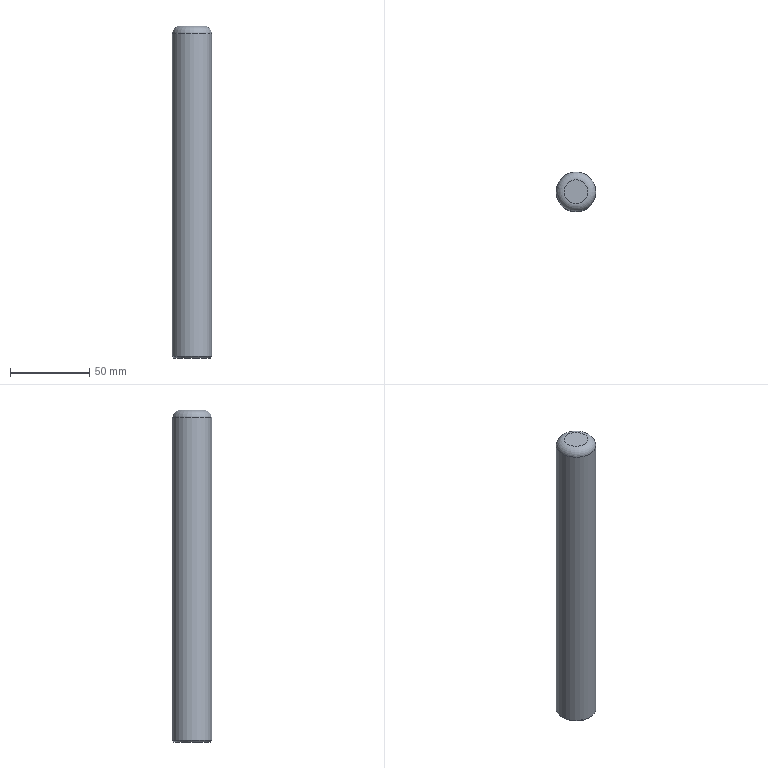Part | STEP file | 200 mesh_id66_xmt | 1 solid | 5 faces | box 25 x 25 x 210 mm | volume 102662 mm3 | plane 2 | cylinder 1 | cone 1 | torus 1 | commonest cylinder face diameters 25 x1
STEP:
#1=CARTESIAN_POINT('',(-17045.384,-4158.269,160.));
#2=VERTEX_POINT('',#1);
#3=CARTESIAN_POINT('',(-17052.884,-4158.269,160.));
#4=DIRECTION('',(0.,0.,1.));
#5=DIRECTION('',(1.,0.,0.));
#6=AXIS2_PLACEMENT_3D('',#3,#4,#5);
#7=CIRCLE('',#6,7.5);
#8=EDGE_CURVE('',#2,#2,#7,.T.);
#9=ORIENTED_EDGE('',*,*,#8,.T.);
#10=EDGE_LOOP('',(#9));
#11=FACE_OUTER_BOUND('',#10,.T.);
#12=CARTESIAN_POINT('',(-17052.884,-4158.269,160.));
#13=DIRECTION('',(0.,0.,1.));
#14=DIRECTION('',(1.,0.,0.));
#15=AXIS2_PLACEMENT_3D('',#12,#13,#14);
#16=PLANE('',#15);
#17=ADVANCED_FACE('',(#11),#16,.T.);
#18=CARTESIAN_POINT('',(-17064.384,-4158.269,-50.));
#19=VERTEX_POINT('',#18);
#20=CARTESIAN_POINT('',(-17052.884,-4158.269,-50.));
#21=DIRECTION('',(0.,0.,-1.));
#22=DIRECTION('',(-1.,0.,0.));
#23=AXIS2_PLACEMENT_3D('',#20,#21,#22);
#24=CIRCLE('',#23,11.5);
#25=EDGE_CURVE('',#19,#19,#24,.T.);
#26=ORIENTED_EDGE('',*,*,#25,.T.);
#27=EDGE_LOOP('',(#26));
#28=FACE_OUTER_BOUND('',#27,.T.);
#29=CARTESIAN_POINT('',(-17052.884,-4158.269,-50.));
#30=DIRECTION('',(0.,0.,-1.));
#31=DIRECTION('',(-1.,0.,0.));
#32=AXIS2_PLACEMENT_3D('',#29,#30,#31);
#33=PLANE('',#32);
#34=ADVANCED_FACE('',(#28),#33,.T.);
#35=CARTESIAN_POINT('',(-17040.384,-4158.269,155.));
#36=VERTEX_POINT('',#35);
#37=CARTESIAN_POINT('',(-17052.884,-4158.269,155.));
#38=DIRECTION('',(0.,0.,-1.));
#39=DIRECTION('',(1.,0.,0.));
#40=AXIS2_PLACEMENT_3D('',#37,#38,#39);
#41=CIRCLE('',#40,12.5);
#42=EDGE_CURVE('',#36,#36,#41,.T.);
#43=ORIENTED_EDGE('',*,*,#42,.T.);
#44=EDGE_LOOP('',(#43));
#45=FACE_BOUND('',#44,.T.);
#46=CARTESIAN_POINT('',(-17065.384,-4158.269,-49.));
#47=VERTEX_POINT('',#46);
#48=CARTESIAN_POINT('',(-17052.884,-4158.269,-49.));
#49=DIRECTION('',(0.,0.,1.));
#50=DIRECTION('',(-1.,0.,0.));
#51=AXIS2_PLACEMENT_3D('',#48,#49,#50);
#52=CIRCLE('',#51,12.5);
#53=EDGE_CURVE('',#47,#47,#52,.T.);
#54=ORIENTED_EDGE('',*,*,#53,.T.);
#55=EDGE_LOOP('',(#54));
#56=FACE_BOUND('',#55,.T.);
#57=CARTESIAN_POINT('',(-17052.884,-4158.269,-50.));
#58=DIRECTION('',(0.,0.,1.));
#59=DIRECTION('',(1.,0.,0.));
#60=AXIS2_PLACEMENT_3D('',#57,#58,#59);
#61=CYLINDRICAL_SURFACE('',#60,12.5);
#62=ADVANCED_FACE('',(#45,#56),#61,.T.);
#63=ORIENTED_EDGE('',*,*,#25,.F.);
#64=EDGE_LOOP('',(#63));
#65=FACE_BOUND('',#64,.T.);
#66=ORIENTED_EDGE('',*,*,#53,.F.);
#67=EDGE_LOOP('',(#66));
#68=FACE_BOUND('',#67,.T.);
#69=CARTESIAN_POINT('',(-17052.884,-4158.269,-49.));
#70=DIRECTION('',(0.,0.,1.));
#71=DIRECTION('',(1.,0.,0.));
#72=AXIS2_PLACEMENT_3D('',#69,#70,#71);
#73=CONICAL_SURFACE('',#72,12.5,45.);
#74=ADVANCED_FACE('',(#65,#68),#73,.T.);
#75=ORIENTED_EDGE('',*,*,#8,.F.);
#76=EDGE_LOOP('',(#75));
#77=FACE_BOUND('',#76,.T.);
#78=ORIENTED_EDGE('',*,*,#42,.F.);
#79=EDGE_LOOP('',(#78));
#80=FACE_BOUND('',#79,.T.);
#81=CARTESIAN_POINT('',(-17052.884,-4158.269,155.));
#82=DIRECTION('',(0.,0.,1.));
#83=DIRECTION('',(1.,0.,0.));
#84=AXIS2_PLACEMENT_3D('',#81,#82,#83);
#85=TOROIDAL_SURFACE('',#84,7.5,5.);
#86=ADVANCED_FACE('',(#77,#80),#85,.T.);
#87=CLOSED_SHELL('',(#17,#34,#62,#74,#86));
#88=MANIFOLD_SOLID_BREP('',#87);
#89=(LENGTH_UNIT()NAMED_UNIT(*)SI_UNIT(.MILLI.,.METRE.));
#90=UNCERTAINTY_MEASURE_WITH_UNIT(LENGTH_MEASURE(0.00002),#89,'','');
#91=(NAMED_UNIT(*)PLANE_ANGLE_UNIT()SI_UNIT($,.RADIAN.));
#92=PLANE_ANGLE_MEASURE_WITH_UNIT(PLANE_ANGLE_MEASURE(0.01745),#91);
#93=DIMENSIONAL_EXPONENTS(0.,0.,0.,0.,0.,0.,0.);
#94=(CONVERSION_BASED_UNIT('DEGREE',#92)NAMED_UNIT(#93)PLANE_ANGLE_UNIT());
#95=(NAMED_UNIT(*)SI_UNIT($,.STERADIAN.)SOLID_ANGLE_UNIT());
#96=(GEOMETRIC_REPRESENTATION_CONTEXT(3)GLOBAL_UNCERTAINTY_ASSIGNED_CONTEXT((#90))GLOBAL_UNIT_ASSIGNED_CONTEXT((#89,#94,#95))REPRESENTATION_CONTEXT('',''));
#97=ADVANCED_BREP_SHAPE_REPRESENTATION('',(#88),#96);